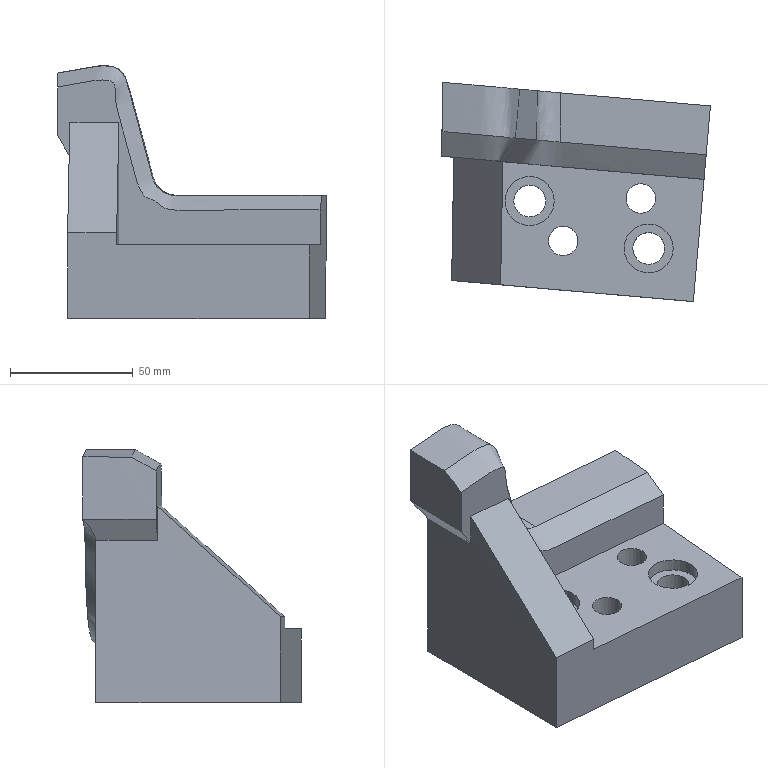Part | NX | features solid 2 | 1 solid | 26 faces | box 109.578 x 89.242 x 103.18 mm | volume 347303 mm3 | spline 11 | plane 9 | cylinder 6 | commonest cylinder face diameters 12 x2 13 x2 20 x2